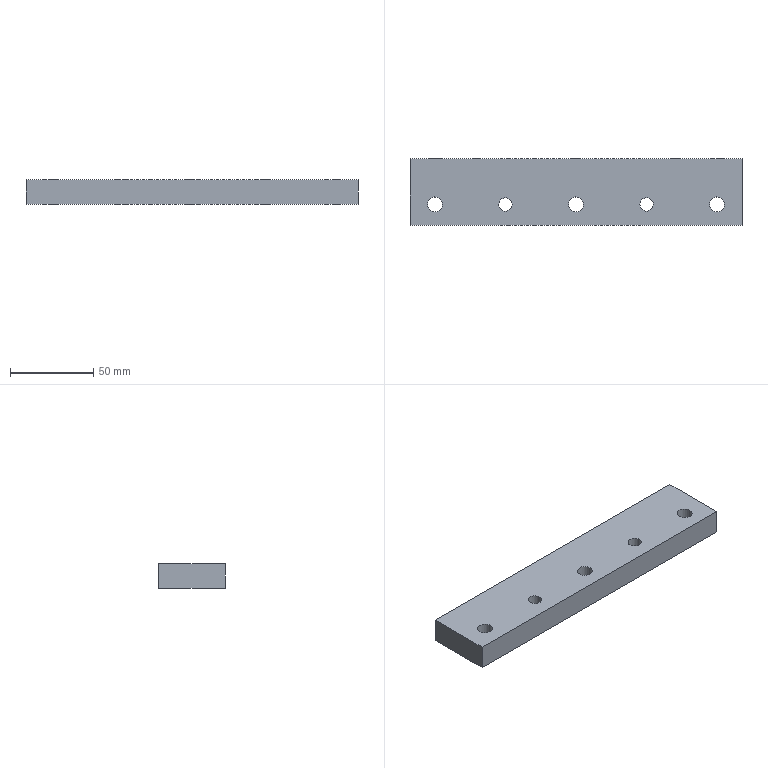Part | STEP file | SN10_001_002_SUPORTE | 1 solid | 21 faces | box 200 x 40 x 15 mm | volume 112660 mm3 | cylinder 10 | plane 6 | cone 5 | commonest cylinder face diameters 8 x4 4.917 x3 9 x3
STEP:
#1=CARTESIAN_POINT('',(0.,0.,0.));
#2=DIRECTION('',(0.,0.,1.));
#3=DIRECTION('',(1.,0.,0.));
#4=AXIS2_PLACEMENT_3D('',#1,#2,#3);
#5=CARTESIAN_POINT('',(-81.49,195.,59.418));
#6=VERTEX_POINT('',#5);
#7=CARTESIAN_POINT('',(-85.,195.,57.5));
#8=DIRECTION('',(0.,1.,0.));
#9=DIRECTION('',(1.,0.,0.));
#10=AXIS2_PLACEMENT_3D('',#7,#8,#9);
#11=CIRCLE('',#10,4.);
#12=CARTESIAN_POINT('',(-85.,193.268,57.5));
#13=DIRECTION('',(0.,1.,0.));
#14=DIRECTION('',(0.8776,0.,0.4794));
#15=AXIS2_PLACEMENT_3D('',#12,#13,#14);
#16=CONICAL_SURFACE('',#15,1.,1.047);
#17=CARTESIAN_POINT('',(-5.783,1.732));
#18=DIRECTION('',(1.,0.));
#19=VECTOR('',#18,1.);
#20=LINE('',#17,#19);
#21=(GEOMETRIC_REPRESENTATION_CONTEXT(2)PARAMETRIC_REPRESENTATION_CONTEXT()REPRESENTATION_CONTEXT('',''));
#22=DEFINITIONAL_REPRESENTATION('',(#20),#21);
#23=PCURVE('',#16,#22);
#24=CARTESIAN_POINT('',(-85.,214.9,57.5));
#25=DIRECTION('',(0.,-1.,0.));
#26=DIRECTION('',(0.8776,0.,0.4794));
#27=AXIS2_PLACEMENT_3D('',#24,#25,#26);
#28=CYLINDRICAL_SURFACE('',#27,4.);
#29=CARTESIAN_POINT('',(12.066,19.9));
#30=DIRECTION('',(-1.,0.));
#31=VECTOR('',#30,1.);
#32=LINE('',#29,#31);
#33=(GEOMETRIC_REPRESENTATION_CONTEXT(2)PARAMETRIC_REPRESENTATION_CONTEXT()REPRESENTATION_CONTEXT('',''));
#34=DEFINITIONAL_REPRESENTATION('',(#32),#33);
#35=PCURVE('',#28,#34);
#36=SURFACE_CURVE('',#11,(#23,#35),.PCURVE_S1.);
#37=EDGE_CURVE('',#6,#6,#36,.T.);
#38=ORIENTED_EDGE('',*,*,#37,.F.);
#39=CARTESIAN_POINT('',(-85.,192.691,57.5));
#40=VERTEX_POINT('',#39);
#41=CARTESIAN_POINT('',(-85.,192.691,57.5));
#42=CARTESIAN_POINT('',(-81.49,195.,59.418));
#43=B_SPLINE_CURVE_WITH_KNOTS('',1,(#41,#42),.UNSPECIFIED.,.F.,.F.,(2,2),(-1.155,3.464),.PIECEWISE_BEZIER_KNOTS.);
#44=CARTESIAN_POINT('',(0.,0.));
#45=DIRECTION('',(0.,1.));
#46=VECTOR('',#45,1.);
#47=LINE('',#44,#46);
#48=(GEOMETRIC_REPRESENTATION_CONTEXT(2)PARAMETRIC_REPRESENTATION_CONTEXT()REPRESENTATION_CONTEXT('',''));
#49=DEFINITIONAL_REPRESENTATION('',(#47),#48);
#50=PCURVE('',#16,#49);
#51=CARTESIAN_POINT('',(6.283,0.));
#52=DIRECTION('',(0.,1.));
#53=VECTOR('',#52,1.);
#54=LINE('',#51,#53);
#55=(GEOMETRIC_REPRESENTATION_CONTEXT(2)PARAMETRIC_REPRESENTATION_CONTEXT()REPRESENTATION_CONTEXT('',''));
#56=DEFINITIONAL_REPRESENTATION('',(#54),#55);
#57=PCURVE('',#16,#56);
#58=SEAM_CURVE('',#43,(#50,#57),.PCURVE_S1.);
#59=EDGE_CURVE('',#40,#6,#58,.T.);
#60=ORIENTED_EDGE('',*,*,#59,.F.);
#61=ORIENTED_EDGE('',*,*,#59,.T.);
#62=EDGE_LOOP('',(#38,#60,#61));
#63=FACE_BOUND('',#62,.F.);
#64=ADVANCED_FACE('',(#63),#16,.F.);
#65=CARTESIAN_POINT('',(-100.,215.,65.));
#66=VERTEX_POINT('',#65);
#67=CARTESIAN_POINT('',(100.,215.,65.));
#68=VERTEX_POINT('',#67);
#69=CARTESIAN_POINT('',(-100.,215.,65.));
#70=DIRECTION('',(1.,0.,0.));
#71=VECTOR('',#70,1.);
#72=LINE('',#69,#71);
#73=CARTESIAN_POINT('',(0.,175.,65.));
#74=DIRECTION('',(0.,0.,-1.));
#75=DIRECTION('',(-1.,0.,0.));
#76=AXIS2_PLACEMENT_3D('',#73,#74,#75);
#77=PLANE('',#76);
#78=CARTESIAN_POINT('',(100.,40.));
#79=DIRECTION('',(-1.,0.));
#80=VECTOR('',#79,1.);
#81=LINE('',#78,#80);
#82=(GEOMETRIC_REPRESENTATION_CONTEXT(2)PARAMETRIC_REPRESENTATION_CONTEXT()REPRESENTATION_CONTEXT('',''));
#83=DEFINITIONAL_REPRESENTATION('',(#81),#82);
#84=PCURVE('',#77,#83);
#85=CARTESIAN_POINT('',(0.,215.,65.));
#86=DIRECTION('',(0.,-1.,0.));
#87=DIRECTION('',(0.,0.,-1.));
#88=AXIS2_PLACEMENT_3D('',#85,#86,#87);
#89=PLANE('',#88);
#90=CARTESIAN_POINT('',(0.,-100.));
#91=DIRECTION('',(0.,1.));
#92=VECTOR('',#91,1.);
#93=LINE('',#90,#92);
#94=(GEOMETRIC_REPRESENTATION_CONTEXT(2)PARAMETRIC_REPRESENTATION_CONTEXT()REPRESENTATION_CONTEXT('',''));
#95=DEFINITIONAL_REPRESENTATION('',(#93),#94);
#96=PCURVE('',#89,#95);
#97=SURFACE_CURVE('',#72,(#84,#96),.PCURVE_S1.);
#98=EDGE_CURVE('',#66,#68,#97,.T.);
#99=ORIENTED_EDGE('',*,*,#98,.F.);
#100=CARTESIAN_POINT('',(-100.,175.,65.));
#101=VERTEX_POINT('',#100);
#102=CARTESIAN_POINT('',(-100.,175.,65.));
#103=DIRECTION('',(0.,1.,0.));
#104=VECTOR('',#103,1.);
#105=LINE('',#102,#104);
#106=CARTESIAN_POINT('',(100.,0.));
#107=DIRECTION('',(0.,1.));
#108=VECTOR('',#107,1.);
#109=LINE('',#106,#108);
#110=(GEOMETRIC_REPRESENTATION_CONTEXT(2)PARAMETRIC_REPRESENTATION_CONTEXT()REPRESENTATION_CONTEXT('',''));
#111=DEFINITIONAL_REPRESENTATION('',(#109),#110);
#112=PCURVE('',#77,#111);
#113=CARTESIAN_POINT('',(-100.,0.,0.));
#114=DIRECTION('',(1.,0.,0.));
#115=DIRECTION('',(0.,0.,-1.));
#116=AXIS2_PLACEMENT_3D('',#113,#114,#115);
#117=PLANE('',#116);
#118=CARTESIAN_POINT('',(-65.,175.));
#119=DIRECTION('',(0.,1.));
#120=VECTOR('',#119,1.);
#121=LINE('',#118,#120);
#122=(GEOMETRIC_REPRESENTATION_CONTEXT(2)PARAMETRIC_REPRESENTATION_CONTEXT()REPRESENTATION_CONTEXT('',''));
#123=DEFINITIONAL_REPRESENTATION('',(#121),#122);
#124=PCURVE('',#117,#123);
#125=SURFACE_CURVE('',#105,(#112,#124),.PCURVE_S1.);
#126=EDGE_CURVE('',#101,#66,#125,.T.);
#127=ORIENTED_EDGE('',*,*,#126,.F.);
#128=CARTESIAN_POINT('',(100.,175.,65.));
#129=VERTEX_POINT('',#128);
#130=CARTESIAN_POINT('',(-100.,175.,65.));
#131=DIRECTION('',(1.,0.,0.));
#132=VECTOR('',#131,1.);
#133=LINE('',#130,#132);
#134=CARTESIAN_POINT('',(100.,0.));
#135=DIRECTION('',(-1.,0.));
#136=VECTOR('',#135,1.);
#137=LINE('',#134,#136);
#138=(GEOMETRIC_REPRESENTATION_CONTEXT(2)PARAMETRIC_REPRESENTATION_CONTEXT()REPRESENTATION_CONTEXT('',''));
#139=DEFINITIONAL_REPRESENTATION('',(#137),#138);
#140=PCURVE('',#77,#139);
#141=CARTESIAN_POINT('',(0.,175.,50.));
#142=DIRECTION('',(0.,1.,0.));
#143=DIRECTION('',(0.,0.,1.));
#144=AXIS2_PLACEMENT_3D('',#141,#142,#143);
#145=PLANE('',#144);
#146=CARTESIAN_POINT('',(15.,-100.));
#147=DIRECTION('',(0.,1.));
#148=VECTOR('',#147,1.);
#149=LINE('',#146,#148);
#150=(GEOMETRIC_REPRESENTATION_CONTEXT(2)PARAMETRIC_REPRESENTATION_CONTEXT()REPRESENTATION_CONTEXT('',''));
#151=DEFINITIONAL_REPRESENTATION('',(#149),#150);
#152=PCURVE('',#145,#151);
#153=SURFACE_CURVE('',#133,(#140,#152),.PCURVE_S1.);
#154=EDGE_CURVE('',#101,#129,#153,.T.);
#155=ORIENTED_EDGE('',*,*,#154,.T.);
#156=CARTESIAN_POINT('',(100.,175.,65.));
#157=DIRECTION('',(0.,1.,0.));
#158=VECTOR('',#157,1.);
#159=LINE('',#156,#158);
#160=CARTESIAN_POINT('',(-100.,0.));
#161=DIRECTION('',(0.,1.));
#162=VECTOR('',#161,1.);
#163=LINE('',#160,#162);
#164=(GEOMETRIC_REPRESENTATION_CONTEXT(2)PARAMETRIC_REPRESENTATION_CONTEXT()REPRESENTATION_CONTEXT('',''));
#165=DEFINITIONAL_REPRESENTATION('',(#163),#164);
#166=PCURVE('',#77,#165);
#167=CARTESIAN_POINT('',(100.,0.,0.));
#168=DIRECTION('',(1.,0.,0.));
#169=DIRECTION('',(0.,0.,-1.));
#170=AXIS2_PLACEMENT_3D('',#167,#168,#169);
#171=PLANE('',#170);
#172=CARTESIAN_POINT('',(-65.,175.));
#173=DIRECTION('',(0.,1.));
#174=VECTOR('',#173,1.);
#175=LINE('',#172,#174);
#176=(GEOMETRIC_REPRESENTATION_CONTEXT(2)PARAMETRIC_REPRESENTATION_CONTEXT()REPRESENTATION_CONTEXT('',''));
#177=DEFINITIONAL_REPRESENTATION('',(#175),#176);
#178=PCURVE('',#171,#177);
#179=SURFACE_CURVE('',#159,(#166,#178),.PCURVE_S1.);
#180=EDGE_CURVE('',#129,#68,#179,.T.);
#181=ORIENTED_EDGE('',*,*,#180,.T.);
#182=EDGE_LOOP('',(#99,#127,#155,#181));
#183=FACE_BOUND('',#182,.T.);
#184=CARTESIAN_POINT('',(38.99,189.418,65.));
#185=VERTEX_POINT('',#184);
#186=CARTESIAN_POINT('',(42.5,187.5,65.));
#187=DIRECTION('',(0.,0.,-1.));
#188=DIRECTION('',(1.,0.,0.));
#189=AXIS2_PLACEMENT_3D('',#186,#187,#188);
#190=CIRCLE('',#189,4.);
#191=CARTESIAN_POINT('',(-42.5,12.5));
#192=DIRECTION('',(-1.,0.));
#193=AXIS2_PLACEMENT_2D('',#191,#192);
#194=CIRCLE('',#193,4.);
#195=(GEOMETRIC_REPRESENTATION_CONTEXT(2)PARAMETRIC_REPRESENTATION_CONTEXT()REPRESENTATION_CONTEXT('',''));
#196=DEFINITIONAL_REPRESENTATION('',(#194),#195);
#197=PCURVE('',#77,#196);
#198=CARTESIAN_POINT('',(42.5,187.5,64.9));
#199=DIRECTION('',(0.,0.,-1.));
#200=DIRECTION('',(0.8776,-0.4794,0.));
#201=AXIS2_PLACEMENT_3D('',#198,#199,#200);
#202=CYLINDRICAL_SURFACE('',#201,4.);
#203=CARTESIAN_POINT('',(-0.5,-0.1));
#204=DIRECTION('',(1.,0.));
#205=VECTOR('',#204,1.);
#206=LINE('',#203,#205);
#207=(GEOMETRIC_REPRESENTATION_CONTEXT(2)PARAMETRIC_REPRESENTATION_CONTEXT()REPRESENTATION_CONTEXT('',''));
#208=DEFINITIONAL_REPRESENTATION('',(#206),#207);
#209=PCURVE('',#202,#208);
#210=SURFACE_CURVE('',#190,(#197,#209),.PCURVE_S1.);
#211=EDGE_CURVE('',#185,#185,#210,.T.);
#212=ORIENTED_EDGE('',*,*,#211,.T.);
#213=EDGE_LOOP('',(#212));
#214=FACE_BOUND('',#213,.T.);
#215=CARTESIAN_POINT('',(-46.01,189.418,65.));
#216=VERTEX_POINT('',#215);
#217=CARTESIAN_POINT('',(-42.5,187.5,65.));
#218=DIRECTION('',(0.,0.,-1.));
#219=DIRECTION('',(1.,0.,0.));
#220=AXIS2_PLACEMENT_3D('',#217,#218,#219);
#221=CIRCLE('',#220,4.);
#222=CARTESIAN_POINT('',(42.5,12.5));
#223=DIRECTION('',(-1.,0.));
#224=AXIS2_PLACEMENT_2D('',#222,#223);
#225=CIRCLE('',#224,4.);
#226=(GEOMETRIC_REPRESENTATION_CONTEXT(2)PARAMETRIC_REPRESENTATION_CONTEXT()REPRESENTATION_CONTEXT('',''));
#227=DEFINITIONAL_REPRESENTATION('',(#225),#226);
#228=PCURVE('',#77,#227);
#229=CARTESIAN_POINT('',(-42.5,187.5,64.9));
#230=DIRECTION('',(0.,0.,-1.));
#231=DIRECTION('',(0.8776,-0.4794,0.));
#232=AXIS2_PLACEMENT_3D('',#229,#230,#231);
#233=CYLINDRICAL_SURFACE('',#232,4.);
#234=CARTESIAN_POINT('',(-0.5,-0.1));
#235=DIRECTION('',(1.,0.));
#236=VECTOR('',#235,1.);
#237=LINE('',#234,#236);
#238=(GEOMETRIC_REPRESENTATION_CONTEXT(2)PARAMETRIC_REPRESENTATION_CONTEXT()REPRESENTATION_CONTEXT('',''));
#239=DEFINITIONAL_REPRESENTATION('',(#237),#238);
#240=PCURVE('',#233,#239);
#241=SURFACE_CURVE('',#221,(#228,#240),.PCURVE_S1.);
#242=EDGE_CURVE('',#216,#216,#241,.T.);
#243=ORIENTED_EDGE('',*,*,#242,.T.);
#244=EDGE_LOOP('',(#243));
#245=FACE_BOUND('',#244,.T.);
#246=CARTESIAN_POINT('',(-88.949,189.657,65.));
#247=VERTEX_POINT('',#246);
#248=CARTESIAN_POINT('',(-85.,187.5,65.));
#249=DIRECTION('',(0.,0.,-1.));
#250=DIRECTION('',(1.,0.,0.));
#251=AXIS2_PLACEMENT_3D('',#248,#249,#250);
#252=CIRCLE('',#251,4.5);
#253=CARTESIAN_POINT('',(85.,12.5));
#254=DIRECTION('',(-1.,0.));
#255=AXIS2_PLACEMENT_2D('',#253,#254);
#256=CIRCLE('',#255,4.5);
#257=(GEOMETRIC_REPRESENTATION_CONTEXT(2)PARAMETRIC_REPRESENTATION_CONTEXT()REPRESENTATION_CONTEXT('',''));
#258=DEFINITIONAL_REPRESENTATION('',(#256),#257);
#259=PCURVE('',#77,#258);
#260=CARTESIAN_POINT('',(-85.,187.5,64.9));
#261=DIRECTION('',(0.,0.,-1.));
#262=DIRECTION('',(0.8776,-0.4794,0.));
#263=AXIS2_PLACEMENT_3D('',#260,#261,#262);
#264=CYLINDRICAL_SURFACE('',#263,4.5);
#265=CARTESIAN_POINT('',(-0.5,-0.1));
#266=DIRECTION('',(1.,0.));
#267=VECTOR('',#266,1.);
#268=LINE('',#265,#267);
#269=(GEOMETRIC_REPRESENTATION_CONTEXT(2)PARAMETRIC_REPRESENTATION_CONTEXT()REPRESENTATION_CONTEXT('',''));
#270=DEFINITIONAL_REPRESENTATION('',(#268),#269);
#271=PCURVE('',#264,#270);
#272=SURFACE_CURVE('',#252,(#259,#271),.PCURVE_S1.);
#273=EDGE_CURVE('',#247,#247,#272,.T.);
#274=ORIENTED_EDGE('',*,*,#273,.T.);
#275=EDGE_LOOP('',(#274));
#276=FACE_BOUND('',#275,.T.);
#277=CARTESIAN_POINT('',(-3.949,189.657,65.));
#278=VERTEX_POINT('',#277);
#279=CARTESIAN_POINT('',(0.,187.5,65.));
#280=DIRECTION('',(0.,0.,-1.));
#281=DIRECTION('',(1.,0.,0.));
#282=AXIS2_PLACEMENT_3D('',#279,#280,#281);
#283=CIRCLE('',#282,4.5);
#284=CARTESIAN_POINT('',(0.,12.5));
#285=DIRECTION('',(-1.,0.));
#286=AXIS2_PLACEMENT_2D('',#284,#285);
#287=CIRCLE('',#286,4.5);
#288=(GEOMETRIC_REPRESENTATION_CONTEXT(2)PARAMETRIC_REPRESENTATION_CONTEXT()REPRESENTATION_CONTEXT('',''));
#289=DEFINITIONAL_REPRESENTATION('',(#287),#288);
#290=PCURVE('',#77,#289);
#291=CARTESIAN_POINT('',(0.,187.5,64.9));
#292=DIRECTION('',(0.,0.,-1.));
#293=DIRECTION('',(0.8776,-0.4794,0.));
#294=AXIS2_PLACEMENT_3D('',#291,#292,#293);
#295=CYLINDRICAL_SURFACE('',#294,4.5);
#296=CARTESIAN_POINT('',(-0.5,-0.1));
#297=DIRECTION('',(1.,0.));
#298=VECTOR('',#297,1.);
#299=LINE('',#296,#298);
#300=(GEOMETRIC_REPRESENTATION_CONTEXT(2)PARAMETRIC_REPRESENTATION_CONTEXT()REPRESENTATION_CONTEXT('',''));
#301=DEFINITIONAL_REPRESENTATION('',(#299),#300);
#302=PCURVE('',#295,#301);
#303=SURFACE_CURVE('',#283,(#290,#302),.PCURVE_S1.);
#304=EDGE_CURVE('',#278,#278,#303,.T.);
#305=ORIENTED_EDGE('',*,*,#304,.T.);
#306=EDGE_LOOP('',(#305));
#307=FACE_BOUND('',#306,.T.);
#308=CARTESIAN_POINT('',(81.051,189.657,65.));
#309=VERTEX_POINT('',#308);
#310=CARTESIAN_POINT('',(85.,187.5,65.));
#311=DIRECTION('',(0.,0.,-1.));
#312=DIRECTION('',(1.,0.,0.));
#313=AXIS2_PLACEMENT_3D('',#310,#311,#312);
#314=CIRCLE('',#313,4.5);
#315=CARTESIAN_POINT('',(-85.,12.5));
#316=DIRECTION('',(-1.,0.));
#317=AXIS2_PLACEMENT_2D('',#315,#316);
#318=CIRCLE('',#317,4.5);
#319=(GEOMETRIC_REPRESENTATION_CONTEXT(2)PARAMETRIC_REPRESENTATION_CONTEXT()REPRESENTATION_CONTEXT('',''));
#320=DEFINITIONAL_REPRESENTATION('',(#318),#319);
#321=PCURVE('',#77,#320);
#322=CARTESIAN_POINT('',(85.,187.5,64.9));
#323=DIRECTION('',(0.,0.,-1.));
#324=DIRECTION('',(0.8776,-0.4794,0.));
#325=AXIS2_PLACEMENT_3D('',#322,#323,#324);
#326=CYLINDRICAL_SURFACE('',#325,4.5);
#327=CARTESIAN_POINT('',(-0.5,-0.1));
#328=DIRECTION('',(1.,0.));
#329=VECTOR('',#328,1.);
#330=LINE('',#327,#329);
#331=(GEOMETRIC_REPRESENTATION_CONTEXT(2)PARAMETRIC_REPRESENTATION_CONTEXT()REPRESENTATION_CONTEXT('',''));
#332=DEFINITIONAL_REPRESENTATION('',(#330),#331);
#333=PCURVE('',#326,#332);
#334=SURFACE_CURVE('',#314,(#321,#333),.PCURVE_S1.);
#335=EDGE_CURVE('',#309,#309,#334,.T.);
#336=ORIENTED_EDGE('',*,*,#335,.T.);
#337=EDGE_LOOP('',(#336));
#338=FACE_BOUND('',#337,.T.);
#339=ADVANCED_FACE('',(#183,#214,#245,#276,#307,#338),#77,.F.);
#340=CARTESIAN_POINT('',(-100.,215.,50.));
#341=VERTEX_POINT('',#340);
#342=CARTESIAN_POINT('',(-100.,215.,65.));
#343=DIRECTION('',(0.,0.,-1.));
#344=VECTOR('',#343,1.);
#345=LINE('',#342,#344);
#346=CARTESIAN_POINT('',(-65.,215.));
#347=DIRECTION('',(1.,0.));
#348=VECTOR('',#347,1.);
#349=LINE('',#346,#348);
#350=(GEOMETRIC_REPRESENTATION_CONTEXT(2)PARAMETRIC_REPRESENTATION_CONTEXT()REPRESENTATION_CONTEXT('',''));
#351=DEFINITIONAL_REPRESENTATION('',(#349),#350);
#352=PCURVE('',#117,#351);
#353=CARTESIAN_POINT('',(0.,-100.));
#354=DIRECTION('',(1.,0.));
#355=VECTOR('',#354,1.);
#356=LINE('',#353,#355);
#357=(GEOMETRIC_REPRESENTATION_CONTEXT(2)PARAMETRIC_REPRESENTATION_CONTEXT()REPRESENTATION_CONTEXT('',''));
#358=DEFINITIONAL_REPRESENTATION('',(#356),#357);
#359=PCURVE('',#89,#358);
#360=SURFACE_CURVE('',#345,(#352,#359),.PCURVE_S1.);
#361=EDGE_CURVE('',#66,#341,#360,.T.);
#362=ORIENTED_EDGE('',*,*,#361,.T.);
#363=CARTESIAN_POINT('',(-100.,175.,50.));
#364=VERTEX_POINT('',#363);
#365=CARTESIAN_POINT('',(-100.,215.,50.));
#366=DIRECTION('',(0.,-1.,0.));
#367=VECTOR('',#366,1.);
#368=LINE('',#365,#367);
#369=CARTESIAN_POINT('',(-50.,215.));
#370=DIRECTION('',(0.,-1.));
#371=VECTOR('',#370,1.);
#372=LINE('',#369,#371);
#373=(GEOMETRIC_REPRESENTATION_CONTEXT(2)PARAMETRIC_REPRESENTATION_CONTEXT()REPRESENTATION_CONTEXT('',''));
#374=DEFINITIONAL_REPRESENTATION('',(#372),#373);
#375=PCURVE('',#117,#374);
#376=CARTESIAN_POINT('',(0.,215.,50.));
#377=DIRECTION('',(0.,0.,1.));
#378=DIRECTION('',(1.,0.,0.));
#379=AXIS2_PLACEMENT_3D('',#376,#377,#378);
#380=PLANE('',#379);
#381=CARTESIAN_POINT('',(-100.,0.));
#382=DIRECTION('',(0.,-1.));
#383=VECTOR('',#382,1.);
#384=LINE('',#381,#383);
#385=(GEOMETRIC_REPRESENTATION_CONTEXT(2)PARAMETRIC_REPRESENTATION_CONTEXT()REPRESENTATION_CONTEXT('',''));
#386=DEFINITIONAL_REPRESENTATION('',(#384),#385);
#387=PCURVE('',#380,#386);
#388=SURFACE_CURVE('',#368,(#375,#387),.PCURVE_S1.);
#389=EDGE_CURVE('',#341,#364,#388,.T.);
#390=ORIENTED_EDGE('',*,*,#389,.T.);
#391=CARTESIAN_POINT('',(-100.,175.,50.));
#392=DIRECTION('',(0.,0.,1.));
#393=VECTOR('',#392,1.);
#394=LINE('',#391,#393);
#395=CARTESIAN_POINT('',(-50.,175.));
#396=DIRECTION('',(-1.,0.));
#397=VECTOR('',#396,1.);
#398=LINE('',#395,#397);
#399=(GEOMETRIC_REPRESENTATION_CONTEXT(2)PARAMETRIC_REPRESENTATION_CONTEXT()REPRESENTATION_CONTEXT('',''));
#400=DEFINITIONAL_REPRESENTATION('',(#398),#399);
#401=PCURVE('',#117,#400);
#402=CARTESIAN_POINT('',(0.,-100.));
#403=DIRECTION('',(1.,0.));
#404=VECTOR('',#403,1.);
#405=LINE('',#402,#404);
#406=(GEOMETRIC_REPRESENTATION_CONTEXT(2)PARAMETRIC_REPRESENTATION_CONTEXT()REPRESENTATION_CONTEXT('',''));
#407=DEFINITIONAL_REPRESENTATION('',(#405),#406);
#408=PCURVE('',#145,#407);
#409=SURFACE_CURVE('',#394,(#401,#408),.PCURVE_S1.);
#410=EDGE_CURVE('',#364,#101,#409,.T.);
#411=ORIENTED_EDGE('',*,*,#410,.T.);
#412=ORIENTED_EDGE('',*,*,#126,.T.);
#413=EDGE_LOOP('',(#362,#390,#411,#412));
#414=FACE_BOUND('',#413,.T.);
#415=ADVANCED_FACE('',(#414),#117,.F.);
#416=CARTESIAN_POINT('',(81.49,215.,55.582));
#417=VERTEX_POINT('',#416);
#418=CARTESIAN_POINT('',(85.,215.,57.5));
#419=DIRECTION('',(0.,-1.,0.));
#420=DIRECTION('',(1.,0.,0.));
#421=AXIS2_PLACEMENT_3D('',#418,#419,#420);
#422=CIRCLE('',#421,4.);
#423=CARTESIAN_POINT('',(85.,214.9,57.5));
#424=DIRECTION('',(0.,-1.,0.));
#425=DIRECTION('',(0.8776,0.,0.4794));
#426=AXIS2_PLACEMENT_3D('',#423,#424,#425);
#427=CYLINDRICAL_SURFACE('',#426,4.);
#428=CARTESIAN_POINT('',(-0.5,-0.1));
#429=DIRECTION('',(1.,0.));
#430=VECTOR('',#429,1.);
#431=LINE('',#428,#430);
#432=(GEOMETRIC_REPRESENTATION_CONTEXT(2)PARAMETRIC_REPRESENTATION_CONTEXT()REPRESENTATION_CONTEXT('',''));
#433=DEFINITIONAL_REPRESENTATION('',(#431),#432);
#434=PCURVE('',#427,#433);
#435=CARTESIAN_POINT('',(7.5,85.));
#436=DIRECTION('',(0.,1.));
#437=AXIS2_PLACEMENT_2D('',#435,#436);
#438=CIRCLE('',#437,4.);
#439=(GEOMETRIC_REPRESENTATION_CONTEXT(2)PARAMETRIC_REPRESENTATION_CONTEXT()REPRESENTATION_CONTEXT('',''));
#440=DEFINITIONAL_REPRESENTATION('',(#438),#439);
#441=PCURVE('',#89,#440);
#442=SURFACE_CURVE('',#422,(#434,#441),.PCURVE_S1.);
#443=EDGE_CURVE('',#417,#417,#442,.T.);
#444=ORIENTED_EDGE('',*,*,#443,.T.);
#445=CARTESIAN_POINT('',(81.49,195.,55.582));
#446=VERTEX_POINT('',#445);
#447=CARTESIAN_POINT('',(81.49,215.,55.582));
#448=CARTESIAN_POINT('',(81.49,195.,55.582));
#449=B_SPLINE_CURVE_WITH_KNOTS('',1,(#447,#448),.UNSPECIFIED.,.F.,.F.,(2,2),(-0.1,19.9),.PIECEWISE_BEZIER_KNOTS.);
#450=CARTESIAN_POINT('',(9.425,0.));
#451=DIRECTION('',(0.,1.));
#452=VECTOR('',#451,1.);
#453=LINE('',#450,#452);
#454=(GEOMETRIC_REPRESENTATION_CONTEXT(2)PARAMETRIC_REPRESENTATION_CONTEXT()REPRESENTATION_CONTEXT('',''));
#455=DEFINITIONAL_REPRESENTATION('',(#453),#454);
#456=PCURVE('',#427,#455);
#457=CARTESIAN_POINT('',(3.142,0.));
#458=DIRECTION('',(0.,1.));
#459=VECTOR('',#458,1.);
#460=LINE('',#457,#459);
#461=(GEOMETRIC_REPRESENTATION_CONTEXT(2)PARAMETRIC_REPRESENTATION_CONTEXT()REPRESENTATION_CONTEXT('',''));
#462=DEFINITIONAL_REPRESENTATION('',(#460),#461);
#463=PCURVE('',#427,#462);
#464=SEAM_CURVE('',#449,(#456,#463),.PCURVE_S1.);
#465=EDGE_CURVE('',#417,#446,#464,.T.);
#466=ORIENTED_EDGE('',*,*,#465,.T.);
#467=CARTESIAN_POINT('',(85.,195.,57.5));
#468=DIRECTION('',(0.,-1.,0.));
#469=DIRECTION('',(1.,0.,0.));
#470=AXIS2_PLACEMENT_3D('',#467,#468,#469);
#471=CIRCLE('',#470,4.);
#472=CARTESIAN_POINT('',(-0.5,19.9));
#473=DIRECTION('',(1.,0.));
#474=VECTOR('',#473,1.);
#475=LINE('',#472,#474);
#476=(GEOMETRIC_REPRESENTATION_CONTEXT(2)PARAMETRIC_REPRESENTATION_CONTEXT()REPRESENTATION_CONTEXT('',''));
#477=DEFINITIONAL_REPRESENTATION('',(#475),#476);
#478=PCURVE('',#427,#477);
#479=CARTESIAN_POINT('',(85.,193.268,57.5));
#480=DIRECTION('',(0.,1.,0.));
#481=DIRECTION('',(0.8776,0.,0.4794));
#482=AXIS2_PLACEMENT_3D('',#479,#480,#481);
#483=CONICAL_SURFACE('',#482,1.,1.047);
#484=CARTESIAN_POINT('',(13.066,1.732));
#485=DIRECTION('',(-1.,0.));
#486=VECTOR('',#485,1.);
#487=LINE('',#484,#486);
#488=(GEOMETRIC_REPRESENTATION_CONTEXT(2)PARAMETRIC_REPRESENTATION_CONTEXT()REPRESENTATION_CONTEXT('',''));
#489=DEFINITIONAL_REPRESENTATION('',(#487),#488);
#490=PCURVE('',#483,#489);
#491=SURFACE_CURVE('',#471,(#478,#490),.PCURVE_S1.);
#492=EDGE_CURVE('',#446,#446,#491,.T.);
#493=ORIENTED_EDGE('',*,*,#492,.F.);
#494=ORIENTED_EDGE('',*,*,#465,.F.);
#495=EDGE_LOOP('',(#444,#466,#493,#494));
#496=FACE_BOUND('',#495,.F.);
#497=ADVANCED_FACE('',(#496),#427,.F.);
#498=CARTESIAN_POINT('',(-62.158,215.,56.321));
#499=VERTEX_POINT('',#498);
#500=CARTESIAN_POINT('',(-60.,215.,57.5));
#501=DIRECTION('',(0.,-1.,0.));
#502=DIRECTION('',(1.,0.,0.));
#503=AXIS2_PLACEMENT_3D('',#500,#501,#502);
#504=CIRCLE('',#503,2.458);
#505=CARTESIAN_POINT('',(-60.,214.9,57.5));
#506=DIRECTION('',(0.,-1.,0.));
#507=DIRECTION('',(0.8776,0.,0.4794));
#508=AXIS2_PLACEMENT_3D('',#505,#506,#507);
#509=CYLINDRICAL_SURFACE('',#508,2.458);
#510=CARTESIAN_POINT('',(-0.5,-0.1));
#511=DIRECTION('',(1.,0.));
#512=VECTOR('',#511,1.);
#513=LINE('',#510,#512);
#514=(GEOMETRIC_REPRESENTATION_CONTEXT(2)PARAMETRIC_REPRESENTATION_CONTEXT()REPRESENTATION_CONTEXT('',''));
#515=DEFINITIONAL_REPRESENTATION('',(#513),#514);
#516=PCURVE('',#509,#515);
#517=CARTESIAN_POINT('',(7.5,-60.));
#518=DIRECTION('',(0.,1.));
#519=AXIS2_PLACEMENT_2D('',#517,#518);
#520=CIRCLE('',#519,2.458);
#521=(GEOMETRIC_REPRESENTATION_CONTEXT(2)PARAMETRIC_REPRESENTATION_CONTEXT()REPRESENTATION_CONTEXT('',''));
#522=DEFINITIONAL_REPRESENTATION('',(#520),#521);
#523=PCURVE('',#89,#522);
#524=SURFACE_CURVE('',#504,(#516,#523),.PCURVE_S1.);
#525=EDGE_CURVE('',#499,#499,#524,.T.);
#526=ORIENTED_EDGE('',*,*,#525,.T.);
#527=CARTESIAN_POINT('',(-62.158,200.,56.321));
#528=VERTEX_POINT('',#527);
#529=CARTESIAN_POINT('',(-62.158,215.,56.321));
#530=CARTESIAN_POINT('',(-62.158,200.,56.321));
#531=B_SPLINE_CURVE_WITH_KNOTS('',1,(#529,#530),.UNSPECIFIED.,.F.,.F.,(2,2),(-0.1,14.9),.PIECEWISE_BEZIER_KNOTS.);
#532=CARTESIAN_POINT('',(9.425,0.));
#533=DIRECTION('',(0.,1.));
#534=VECTOR('',#533,1.);
#535=LINE('',#532,#534);
#536=(GEOMETRIC_REPRESENTATION_CONTEXT(2)PARAMETRIC_REPRESENTATION_CONTEXT()REPRESENTATION_CONTEXT('',''));
#537=DEFINITIONAL_REPRESENTATION('',(#535),#536);
#538=PCURVE('',#509,#537);
#539=CARTESIAN_POINT('',(3.142,0.));
#540=DIRECTION('',(0.,1.));
#541=VECTOR('',#540,1.);
#542=LINE('',#539,#541);
#543=(GEOMETRIC_REPRESENTATION_CONTEXT(2)PARAMETRIC_REPRESENTATION_CONTEXT()REPRESENTATION_CONTEXT('',''));
#544=DEFINITIONAL_REPRESENTATION('',(#542),#543);
#545=PCURVE('',#509,#544);
#546=SEAM_CURVE('',#531,(#538,#545),.PCURVE_S1.);
#547=EDGE_CURVE('',#499,#528,#546,.T.);
#548=ORIENTED_EDGE('',*,*,#547,.T.);
#549=CARTESIAN_POINT('',(-60.,200.,57.5));
#550=DIRECTION('',(0.,-1.,0.));
#551=DIRECTION('',(1.,0.,0.));
#552=AXIS2_PLACEMENT_3D('',#549,#550,#551);
#553=CIRCLE('',#552,2.458);
#554=CARTESIAN_POINT('',(-0.5,14.9));
#555=DIRECTION('',(1.,0.));
#556=VECTOR('',#555,1.);
#557=LINE('',#554,#556);
#558=(GEOMETRIC_REPRESENTATION_CONTEXT(2)PARAMETRIC_REPRESENTATION_CONTEXT()REPRESENTATION_CONTEXT('',''));
#559=DEFINITIONAL_REPRESENTATION('',(#557),#558);
#560=PCURVE('',#509,#559);
#561=CARTESIAN_POINT('',(-60.,199.158,57.5));
#562=DIRECTION('',(0.,1.,0.));
#563=DIRECTION('',(0.8776,0.,0.4794));
#564=AXIS2_PLACEMENT_3D('',#561,#562,#563);
#565=CONICAL_SURFACE('',#564,1.,1.047);
#566=CARTESIAN_POINT('',(13.066,0.8421));
#567=DIRECTION('',(-1.,0.));
#568=VECTOR('',#567,1.);
#569=LINE('',#566,#568);
#570=(GEOMETRIC_REPRESENTATION_CONTEXT(2)PARAMETRIC_REPRESENTATION_CONTEXT()REPRESENTATION_CONTEXT('',''));
#571=DEFINITIONAL_REPRESENTATION('',(#569),#570);
#572=PCURVE('',#565,#571);
#573=SURFACE_CURVE('',#553,(#560,#572),.PCURVE_S1.);
#574=EDGE_CURVE('',#528,#528,#573,.T.);
#575=ORIENTED_EDGE('',*,*,#574,.F.);
#576=ORIENTED_EDGE('',*,*,#547,.F.);
#577=EDGE_LOOP('',(#526,#548,#575,#576));
#578=FACE_BOUND('',#577,.F.);
#579=ADVANCED_FACE('',(#578),#509,.F.);
#580=CARTESIAN_POINT('',(-2.158,215.,56.321));
#581=VERTEX_POINT('',#580);
#582=CARTESIAN_POINT('',(0.,215.,57.5));
#583=DIRECTION('',(0.,-1.,0.));
#584=DIRECTION('',(1.,0.,0.));
#585=AXIS2_PLACEMENT_3D('',#582,#583,#584);
#586=CIRCLE('',#585,2.458);
#587=CARTESIAN_POINT('',(0.,214.9,57.5));
#588=DIRECTION('',(0.,-1.,0.));
#589=DIRECTION('',(0.8776,0.,0.4794));
#590=AXIS2_PLACEMENT_3D('',#587,#588,#589);
#591=CYLINDRICAL_SURFACE('',#590,2.458);
#592=CARTESIAN_POINT('',(-0.5,-0.1));
#593=DIRECTION('',(1.,0.));
#594=VECTOR('',#593,1.);
#595=LINE('',#592,#594);
#596=(GEOMETRIC_REPRESENTATION_CONTEXT(2)PARAMETRIC_REPRESENTATION_CONTEXT()REPRESENTATION_CONTEXT('',''));
#597=DEFINITIONAL_REPRESENTATION('',(#595),#596);
#598=PCURVE('',#591,#597);
#599=CARTESIAN_POINT('',(7.5,0.));
#600=DIRECTION('',(0.,1.));
#601=AXIS2_PLACEMENT_2D('',#599,#600);
#602=CIRCLE('',#601,2.458);
#603=(GEOMETRIC_REPRESENTATION_CONTEXT(2)PARAMETRIC_REPRESENTATION_CONTEXT()REPRESENTATION_CONTEXT('',''));
#604=DEFINITIONAL_REPRESENTATION('',(#602),#603);
#605=PCURVE('',#89,#604);
#606=SURFACE_CURVE('',#586,(#598,#605),.PCURVE_S1.);
#607=EDGE_CURVE('',#581,#581,#606,.T.);
#608=ORIENTED_EDGE('',*,*,#607,.T.);
#609=CARTESIAN_POINT('',(-2.158,200.,56.321));
#610=VERTEX_POINT('',#609);
#611=CARTESIAN_POINT('',(-2.158,215.,56.321));
#612=CARTESIAN_POINT('',(-2.158,200.,56.321));
#613=B_SPLINE_CURVE_WITH_KNOTS('',1,(#611,#612),.UNSPECIFIED.,.F.,.F.,(2,2),(-0.1,14.9),.PIECEWISE_BEZIER_KNOTS.);
#614=CARTESIAN_POINT('',(9.425,0.));
#615=DIRECTION('',(0.,1.));
#616=VECTOR('',#615,1.);
#617=LINE('',#614,#616);
#618=(GEOMETRIC_REPRESENTATION_CONTEXT(2)PARAMETRIC_REPRESENTATION_CONTEXT()REPRESENTATION_CONTEXT('',''));
#619=DEFINITIONAL_REPRESENTATION('',(#617),#618);
#620=PCURVE('',#591,#619);
#621=CARTESIAN_POINT('',(3.142,0.));
#622=DIRECTION('',(0.,1.));
#623=VECTOR('',#622,1.);
#624=LINE('',#621,#623);
#625=(GEOMETRIC_REPRESENTATION_CONTEXT(2)PARAMETRIC_REPRESENTATION_CONTEXT()REPRESENTATION_CONTEXT('',''));
#626=DEFINITIONAL_REPRESENTATION('',(#624),#625);
#627=PCURVE('',#591,#626);
#628=SEAM_CURVE('',#613,(#620,#627),.PCURVE_S1.);
#629=EDGE_CURVE('',#581,#610,#628,.T.);
#630=ORIENTED_EDGE('',*,*,#629,.T.);
#631=CARTESIAN_POINT('',(0.,200.,57.5));
#632=DIRECTION('',(0.,-1.,0.));
#633=DIRECTION('',(1.,0.,0.));
#634=AXIS2_PLACEMENT_3D('',#631,#632,#633);
#635=CIRCLE('',#634,2.458);
#636=CARTESIAN_POINT('',(-0.5,14.9));
#637=DIRECTION('',(1.,0.));
#638=VECTOR('',#637,1.);
#639=LINE('',#636,#638);
#640=(GEOMETRIC_REPRESENTATION_CONTEXT(2)PARAMETRIC_REPRESENTATION_CONTEXT()REPRESENTATION_CONTEXT('',''));
#641=DEFINITIONAL_REPRESENTATION('',(#639),#640);
#642=PCURVE('',#591,#641);
#643=CARTESIAN_POINT('',(0.,199.158,57.5));
#644=DIRECTION('',(0.,1.,0.));
#645=DIRECTION('',(0.8776,0.,0.4794));
#646=AXIS2_PLACEMENT_3D('',#643,#644,#645);
#647=CONICAL_SURFACE('',#646,1.,1.047);
#648=CARTESIAN_POINT('',(13.066,0.8421));
#649=DIRECTION('',(-1.,0.));
#650=VECTOR('',#649,1.);
#651=LINE('',#648,#650);
#652=(GEOMETRIC_REPRESENTATION_CONTEXT(2)PARAMETRIC_REPRESENTATION_CONTEXT()REPRESENTATION_CONTEXT('',''));
#653=DEFINITIONAL_REPRESENTATION('',(#651),#652);
#654=PCURVE('',#647,#653);
#655=SURFACE_CURVE('',#635,(#642,#654),.PCURVE_S1.);
#656=EDGE_CURVE('',#610,#610,#655,.T.);
#657=ORIENTED_EDGE('',*,*,#656,.F.);
#658=ORIENTED_EDGE('',*,*,#629,.F.);
#659=EDGE_LOOP('',(#608,#630,#657,#658));
#660=FACE_BOUND('',#659,.F.);
#661=ADVANCED_FACE('',(#660),#591,.F.);
#662=CARTESIAN_POINT('',(57.842,215.,56.321));
#663=VERTEX_POINT('',#662);
#664=CARTESIAN_POINT('',(60.,215.,57.5));
#665=DIRECTION('',(0.,-1.,0.));
#666=DIRECTION('',(1.,0.,0.));
#667=AXIS2_PLACEMENT_3D('',#664,#665,#666);
#668=CIRCLE('',#667,2.458);
#669=CARTESIAN_POINT('',(60.,214.9,57.5));
#670=DIRECTION('',(0.,-1.,0.));
#671=DIRECTION('',(0.8776,0.,0.4794));
#672=AXIS2_PLACEMENT_3D('',#669,#670,#671);
#673=CYLINDRICAL_SURFACE('',#672,2.458);
#674=CARTESIAN_POINT('',(-0.5,-0.1));
#675=DIRECTION('',(1.,0.));
#676=VECTOR('',#675,1.);
#677=LINE('',#674,#676);
#678=(GEOMETRIC_REPRESENTATION_CONTEXT(2)PARAMETRIC_REPRESENTATION_CONTEXT()REPRESENTATION_CONTEXT('',''));
#679=DEFINITIONAL_REPRESENTATION('',(#677),#678);
#680=PCURVE('',#673,#679);
#681=CARTESIAN_POINT('',(7.5,60.));
#682=DIRECTION('',(0.,1.));
#683=AXIS2_PLACEMENT_2D('',#681,#682);
#684=CIRCLE('',#683,2.458);
#685=(GEOMETRIC_REPRESENTATION_CONTEXT(2)PARAMETRIC_REPRESENTATION_CONTEXT()REPRESENTATION_CONTEXT('',''));
#686=DEFINITIONAL_REPRESENTATION('',(#684),#685);
#687=PCURVE('',#89,#686);
#688=SURFACE_CURVE('',#668,(#680,#687),.PCURVE_S1.);
#689=EDGE_CURVE('',#663,#663,#688,.T.);
#690=ORIENTED_EDGE('',*,*,#689,.T.);
#691=CARTESIAN_POINT('',(57.842,200.,56.321));
#692=VERTEX_POINT('',#691);
#693=CARTESIAN_POINT('',(57.842,215.,56.321));
#694=CARTESIAN_POINT('',(57.842,200.,56.321));
#695=B_SPLINE_CURVE_WITH_KNOTS('',1,(#693,#694),.UNSPECIFIED.,.F.,.F.,(2,2),(-0.1,14.9),.PIECEWISE_BEZIER_KNOTS.);
#696=CARTESIAN_POINT('',(9.425,0.));
#697=DIRECTION('',(0.,1.));
#698=VECTOR('',#697,1.);
#699=LINE('',#696,#698);
#700=(GEOMETRIC_REPRESENTATION_CONTEXT(2)PARAMETRIC_REPRESENTATION_CONTEXT()REPRESENTATION_CONTEXT('',''));
#701=DEFINITIONAL_REPRESENTATION('',(#699),#700);
#702=PCURVE('',#673,#701);
#703=CARTESIAN_POINT('',(3.142,0.));
#704=DIRECTION('',(0.,1.));
#705=VECTOR('',#704,1.);
#706=LINE('',#703,#705);
#707=(GEOMETRIC_REPRESENTATION_CONTEXT(2)PARAMETRIC_REPRESENTATION_CONTEXT()REPRESENTATION_CONTEXT('',''));
#708=DEFINITIONAL_REPRESENTATION('',(#706),#707);
#709=PCURVE('',#673,#708);
#710=SEAM_CURVE('',#695,(#702,#709),.PCURVE_S1.);
#711=EDGE_CURVE('',#663,#692,#710,.T.);
#712=ORIENTED_EDGE('',*,*,#711,.T.);
#713=CARTESIAN_POINT('',(60.,200.,57.5));
#714=DIRECTION('',(0.,-1.,0.));
#715=DIRECTION('',(1.,0.,0.));
#716=AXIS2_PLACEMENT_3D('',#713,#714,#715);
#717=CIRCLE('',#716,2.458);
#718=CARTESIAN_POINT('',(-0.5,14.9));
#719=DIRECTION('',(1.,0.));
#720=VECTOR('',#719,1.);
#721=LINE('',#718,#720);
#722=(GEOMETRIC_REPRESENTATION_CONTEXT(2)PARAMETRIC_REPRESENTATION_CONTEXT()REPRESENTATION_CONTEXT('',''));
#723=DEFINITIONAL_REPRESENTATION('',(#721),#722);
#724=PCURVE('',#673,#723);
#725=CARTESIAN_POINT('',(60.,199.158,57.5));
#726=DIRECTION('',(0.,1.,0.));
#727=DIRECTION('',(0.8776,0.,0.4794));
#728=AXIS2_PLACEMENT_3D('',#725,#726,#727);
#729=CONICAL_SURFACE('',#728,1.,1.047);
#730=CARTESIAN_POINT('',(13.066,0.8421));
#731=DIRECTION('',(-1.,0.));
#732=VECTOR('',#731,1.);
#733=LINE('',#730,#732);
#734=(GEOMETRIC_REPRESENTATION_CONTEXT(2)PARAMETRIC_REPRESENTATION_CONTEXT()REPRESENTATION_CONTEXT('',''));
#735=DEFINITIONAL_REPRESENTATION('',(#733),#734);
#736=PCURVE('',#729,#735);
#737=SURFACE_CURVE('',#717,(#724,#736),.PCURVE_S1.);
#738=EDGE_CURVE('',#692,#692,#737,.T.);
#739=ORIENTED_EDGE('',*,*,#738,.F.);
#740=ORIENTED_EDGE('',*,*,#711,.F.);
#741=EDGE_LOOP('',(#690,#712,#739,#740));
#742=FACE_BOUND('',#741,.F.);
#743=ADVANCED_FACE('',(#742),#673,.F.);
#744=ORIENTED_EDGE('',*,*,#154,.F.);
#745=ORIENTED_EDGE('',*,*,#410,.F.);
#746=CARTESIAN_POINT('',(100.,175.,50.));
#747=VERTEX_POINT('',#746);
#748=CARTESIAN_POINT('',(-100.,175.,50.));
#749=DIRECTION('',(1.,0.,0.));
#750=VECTOR('',#749,1.);
#751=LINE('',#748,#750);
#752=CARTESIAN_POINT('',(0.,-100.));
#753=DIRECTION('',(0.,1.));
#754=VECTOR('',#753,1.);
#755=LINE('',#752,#754);
#756=(GEOMETRIC_REPRESENTATION_CONTEXT(2)PARAMETRIC_REPRESENTATION_CONTEXT()REPRESENTATION_CONTEXT('',''));
#757=DEFINITIONAL_REPRESENTATION('',(#755),#756);
#758=PCURVE('',#145,#757);
#759=CARTESIAN_POINT('',(-100.,-40.));
#760=DIRECTION('',(1.,0.));
#761=VECTOR('',#760,1.);
#762=LINE('',#759,#761);
#763=(GEOMETRIC_REPRESENTATION_CONTEXT(2)PARAMETRIC_REPRESENTATION_CONTEXT()REPRESENTATION_CONTEXT('',''));
#764=DEFINITIONAL_REPRESENTATION('',(#762),#763);
#765=PCURVE('',#380,#764);
#766=SURFACE_CURVE('',#751,(#758,#765),.PCURVE_S1.);
#767=EDGE_CURVE('',#364,#747,#766,.T.);
#768=ORIENTED_EDGE('',*,*,#767,.T.);
#769=CARTESIAN_POINT('',(100.,175.,50.));
#770=DIRECTION('',(0.,0.,1.));
#771=VECTOR('',#770,1.);
#772=LINE('',#769,#771);
#773=CARTESIAN_POINT('',(0.,100.));
#774=DIRECTION('',(1.,0.));
#775=VECTOR('',#774,1.);
#776=LINE('',#773,#775);
#777=(GEOMETRIC_REPRESENTATION_CONTEXT(2)PARAMETRIC_REPRESENTATION_CONTEXT()REPRESENTATION_CONTEXT('',''));
#778=DEFINITIONAL_REPRESENTATION('',(#776),#777);
#779=PCURVE('',#145,#778);
#780=CARTESIAN_POINT('',(-50.,175.));
#781=DIRECTION('',(-1.,0.));
#782=VECTOR('',#781,1.);
#783=LINE('',#780,#782);
#784=(GEOMETRIC_REPRESENTATION_CONTEXT(2)PARAMETRIC_REPRESENTATION_CONTEXT()REPRESENTATION_CONTEXT('',''));
#785=DEFINITIONAL_REPRESENTATION('',(#783),#784);
#786=PCURVE('',#171,#785);
#787=SURFACE_CURVE('',#772,(#779,#786),.PCURVE_S1.);
#788=EDGE_CURVE('',#747,#129,#787,.T.);
#789=ORIENTED_EDGE('',*,*,#788,.T.);
#790=EDGE_LOOP('',(#744,#745,#768,#789));
#791=FACE_BOUND('',#790,.T.);
#792=ADVANCED_FACE('',(#791),#145,.F.);
#793=ORIENTED_EDGE('',*,*,#211,.T.);
#794=CARTESIAN_POINT('',(38.99,189.418,50.));
#795=VERTEX_POINT('',#794);
#796=CARTESIAN_POINT('',(38.99,189.418,65.));
#797=CARTESIAN_POINT('',(38.99,189.418,50.));
#798=B_SPLINE_CURVE_WITH_KNOTS('',1,(#796,#797),.UNSPECIFIED.,.F.,.F.,(2,2),(-0.1,14.9),.PIECEWISE_BEZIER_KNOTS.);
#799=CARTESIAN_POINT('',(9.425,0.));
#800=DIRECTION('',(0.,1.));
#801=VECTOR('',#800,1.);
#802=LINE('',#799,#801);
#803=(GEOMETRIC_REPRESENTATION_CONTEXT(2)PARAMETRIC_REPRESENTATION_CONTEXT()REPRESENTATION_CONTEXT('',''));
#804=DEFINITIONAL_REPRESENTATION('',(#802),#803);
#805=PCURVE('',#202,#804);
#806=CARTESIAN_POINT('',(3.142,0.));
#807=DIRECTION('',(0.,1.));
#808=VECTOR('',#807,1.);
#809=LINE('',#806,#808);
#810=(GEOMETRIC_REPRESENTATION_CONTEXT(2)PARAMETRIC_REPRESENTATION_CONTEXT()REPRESENTATION_CONTEXT('',''));
#811=DEFINITIONAL_REPRESENTATION('',(#809),#810);
#812=PCURVE('',#202,#811);
#813=SEAM_CURVE('',#798,(#805,#812),.PCURVE_S1.);
#814=EDGE_CURVE('',#185,#795,#813,.T.);
#815=ORIENTED_EDGE('',*,*,#814,.T.);
#816=CARTESIAN_POINT('',(42.5,187.5,50.));
#817=DIRECTION('',(0.,0.,-1.));
#818=DIRECTION('',(1.,0.,0.));
#819=AXIS2_PLACEMENT_3D('',#816,#817,#818);
#820=CIRCLE('',#819,4.);
#821=CARTESIAN_POINT('',(-0.5,14.9));
#822=DIRECTION('',(1.,0.));
#823=VECTOR('',#822,1.);
#824=LINE('',#821,#823);
#825=(GEOMETRIC_REPRESENTATION_CONTEXT(2)PARAMETRIC_REPRESENTATION_CONTEXT()REPRESENTATION_CONTEXT('',''));
#826=DEFINITIONAL_REPRESENTATION('',(#824),#825);
#827=PCURVE('',#202,#826);
#828=CARTESIAN_POINT('',(46.5,-27.5));
#829=CARTESIAN_POINT('',(46.5,-34.428));
#830=CARTESIAN_POINT('',(40.5,-30.964));
#831=CARTESIAN_POINT('',(34.5,-27.5));
#832=CARTESIAN_POINT('',(40.5,-24.036));
#833=CARTESIAN_POINT('',(46.5,-20.572));
#834=CARTESIAN_POINT('',(46.5,-27.5));
#835=(BOUNDED_CURVE()B_SPLINE_CURVE(2,(#828,#829,#830,#831,#832,#833,#834),.UNSPECIFIED.,.T.,.F.)B_SPLINE_CURVE_WITH_KNOTS((1,2,2,2,2,1),(-2.094,0.,2.094,4.189,6.283,8.378),.UNSPECIFIED.)CURVE()GEOMETRIC_REPRESENTATION_ITEM()RATIONAL_B_SPLINE_CURVE((1.,0.5,1.,0.5,1.,0.5,1.))REPRESENTATION_ITEM(''));
#836=(GEOMETRIC_REPRESENTATION_CONTEXT(2)PARAMETRIC_REPRESENTATION_CONTEXT()REPRESENTATION_CONTEXT('',''));
#837=DEFINITIONAL_REPRESENTATION('',(#835),#836);
#838=PCURVE('',#380,#837);
#839=SURFACE_CURVE('',#820,(#827,#838),.PCURVE_S1.);
#840=EDGE_CURVE('',#795,#795,#839,.T.);
#841=ORIENTED_EDGE('',*,*,#840,.F.);
#842=ORIENTED_EDGE('',*,*,#814,.F.);
#843=EDGE_LOOP('',(#793,#815,#841,#842));
#844=FACE_BOUND('',#843,.F.);
#845=ADVANCED_FACE('',(#844),#202,.F.);
#846=ORIENTED_EDGE('',*,*,#242,.T.);
#847=CARTESIAN_POINT('',(-46.01,189.418,50.));
#848=VERTEX_POINT('',#847);
#849=CARTESIAN_POINT('',(-46.01,189.418,65.));
#850=CARTESIAN_POINT('',(-46.01,189.418,50.));
#851=B_SPLINE_CURVE_WITH_KNOTS('',1,(#849,#850),.UNSPECIFIED.,.F.,.F.,(2,2),(-0.1,14.9),.PIECEWISE_BEZIER_KNOTS.);
#852=CARTESIAN_POINT('',(9.425,0.));
#853=DIRECTION('',(0.,1.));
#854=VECTOR('',#853,1.);
#855=LINE('',#852,#854);
#856=(GEOMETRIC_REPRESENTATION_CONTEXT(2)PARAMETRIC_REPRESENTATION_CONTEXT()REPRESENTATION_CONTEXT('',''));
#857=DEFINITIONAL_REPRESENTATION('',(#855),#856);
#858=PCURVE('',#233,#857);
#859=CARTESIAN_POINT('',(3.142,0.));
#860=DIRECTION('',(0.,1.));
#861=VECTOR('',#860,1.);
#862=LINE('',#859,#861);
#863=(GEOMETRIC_REPRESENTATION_CONTEXT(2)PARAMETRIC_REPRESENTATION_CONTEXT()REPRESENTATION_CONTEXT('',''));
#864=DEFINITIONAL_REPRESENTATION('',(#862),#863);
#865=PCURVE('',#233,#864);
#866=SEAM_CURVE('',#851,(#858,#865),.PCURVE_S1.);
#867=EDGE_CURVE('',#216,#848,#866,.T.);
#868=ORIENTED_EDGE('',*,*,#867,.T.);
#869=CARTESIAN_POINT('',(-42.5,187.5,50.));
#870=DIRECTION('',(0.,0.,-1.));
#871=DIRECTION('',(1.,0.,0.));
#872=AXIS2_PLACEMENT_3D('',#869,#870,#871);
#873=CIRCLE('',#872,4.);
#874=CARTESIAN_POINT('',(-0.5,14.9));
#875=DIRECTION('',(1.,0.));
#876=VECTOR('',#875,1.);
#877=LINE('',#874,#876);
#878=(GEOMETRIC_REPRESENTATION_CONTEXT(2)PARAMETRIC_REPRESENTATION_CONTEXT()REPRESENTATION_CONTEXT('',''));
#879=DEFINITIONAL_REPRESENTATION('',(#877),#878);
#880=PCURVE('',#233,#879);
#881=CARTESIAN_POINT('',(-38.5,-27.5));
#882=CARTESIAN_POINT('',(-38.5,-34.428));
#883=CARTESIAN_POINT('',(-44.5,-30.964));
#884=CARTESIAN_POINT('',(-50.5,-27.5));
#885=CARTESIAN_POINT('',(-44.5,-24.036));
#886=CARTESIAN_POINT('',(-38.5,-20.572));
#887=CARTESIAN_POINT('',(-38.5,-27.5));
#888=(BOUNDED_CURVE()B_SPLINE_CURVE(2,(#881,#882,#883,#884,#885,#886,#887),.UNSPECIFIED.,.T.,.F.)B_SPLINE_CURVE_WITH_KNOTS((1,2,2,2,2,1),(-2.094,0.,2.094,4.189,6.283,8.378),.UNSPECIFIED.)CURVE()GEOMETRIC_REPRESENTATION_ITEM()RATIONAL_B_SPLINE_CURVE((1.,0.5,1.,0.5,1.,0.5,1.))REPRESENTATION_ITEM(''));
#889=(GEOMETRIC_REPRESENTATION_CONTEXT(2)PARAMETRIC_REPRESENTATION_CONTEXT()REPRESENTATION_CONTEXT('',''));
#890=DEFINITIONAL_REPRESENTATION('',(#888),#889);
#891=PCURVE('',#380,#890);
#892=SURFACE_CURVE('',#873,(#880,#891),.PCURVE_S1.);
#893=EDGE_CURVE('',#848,#848,#892,.T.);
#894=ORIENTED_EDGE('',*,*,#893,.F.);
#895=ORIENTED_EDGE('',*,*,#867,.F.);
#896=EDGE_LOOP('',(#846,#868,#894,#895));
#897=FACE_BOUND('',#896,.F.);
#898=ADVANCED_FACE('',(#897),#233,.F.);
#899=ORIENTED_EDGE('',*,*,#273,.T.);
#900=CARTESIAN_POINT('',(-88.949,189.657,50.));
#901=VERTEX_POINT('',#900);
#902=CARTESIAN_POINT('',(-88.949,189.657,65.));
#903=CARTESIAN_POINT('',(-88.949,189.657,50.));
#904=B_SPLINE_CURVE_WITH_KNOTS('',1,(#902,#903),.UNSPECIFIED.,.F.,.F.,(2,2),(-0.1,14.9),.PIECEWISE_BEZIER_KNOTS.);
#905=CARTESIAN_POINT('',(9.425,0.));
#906=DIRECTION('',(0.,1.));
#907=VECTOR('',#906,1.);
#908=LINE('',#905,#907);
#909=(GEOMETRIC_REPRESENTATION_CONTEXT(2)PARAMETRIC_REPRESENTATION_CONTEXT()REPRESENTATION_CONTEXT('',''));
#910=DEFINITIONAL_REPRESENTATION('',(#908),#909);
#911=PCURVE('',#264,#910);
#912=CARTESIAN_POINT('',(3.142,0.));
#913=DIRECTION('',(0.,1.));
#914=VECTOR('',#913,1.);
#915=LINE('',#912,#914);
#916=(GEOMETRIC_REPRESENTATION_CONTEXT(2)PARAMETRIC_REPRESENTATION_CONTEXT()REPRESENTATION_CONTEXT('',''));
#917=DEFINITIONAL_REPRESENTATION('',(#915),#916);
#918=PCURVE('',#264,#917);
#919=SEAM_CURVE('',#904,(#911,#918),.PCURVE_S1.);
#920=EDGE_CURVE('',#247,#901,#919,.T.);
#921=ORIENTED_EDGE('',*,*,#920,.T.);
#922=CARTESIAN_POINT('',(-85.,187.5,50.));
#923=DIRECTION('',(0.,0.,-1.));
#924=DIRECTION('',(1.,0.,0.));
#925=AXIS2_PLACEMENT_3D('',#922,#923,#924);
#926=CIRCLE('',#925,4.5);
#927=CARTESIAN_POINT('',(-0.5,14.9));
#928=DIRECTION('',(1.,0.));
#929=VECTOR('',#928,1.);
#930=LINE('',#927,#929);
#931=(GEOMETRIC_REPRESENTATION_CONTEXT(2)PARAMETRIC_REPRESENTATION_CONTEXT()REPRESENTATION_CONTEXT('',''));
#932=DEFINITIONAL_REPRESENTATION('',(#930),#931);
#933=PCURVE('',#264,#932);
#934=CARTESIAN_POINT('',(-80.5,-27.5));
#935=CARTESIAN_POINT('',(-80.5,-35.294));
#936=CARTESIAN_POINT('',(-87.25,-31.397));
#937=CARTESIAN_POINT('',(-94.,-27.5));
#938=CARTESIAN_POINT('',(-87.25,-23.603));
#939=CARTESIAN_POINT('',(-80.5,-19.706));
#940=CARTESIAN_POINT('',(-80.5,-27.5));
#941=(BOUNDED_CURVE()B_SPLINE_CURVE(2,(#934,#935,#936,#937,#938,#939,#940),.UNSPECIFIED.,.T.,.F.)B_SPLINE_CURVE_WITH_KNOTS((1,2,2,2,2,1),(-2.094,0.,2.094,4.189,6.283,8.378),.UNSPECIFIED.)CURVE()GEOMETRIC_REPRESENTATION_ITEM()RATIONAL_B_SPLINE_CURVE((1.,0.5,1.,0.5,1.,0.5,1.))REPRESENTATION_ITEM(''));
#942=(GEOMETRIC_REPRESENTATION_CONTEXT(2)PARAMETRIC_REPRESENTATION_CONTEXT()REPRESENTATION_CONTEXT('',''));
#943=DEFINITIONAL_REPRESENTATION('',(#941),#942);
#944=PCURVE('',#380,#943);
#945=SURFACE_CURVE('',#926,(#933,#944),.PCURVE_S1.);
#946=EDGE_CURVE('',#901,#901,#945,.T.);
#947=ORIENTED_EDGE('',*,*,#946,.F.);
#948=ORIENTED_EDGE('',*,*,#920,.F.);
#949=EDGE_LOOP('',(#899,#921,#947,#948));
#950=FACE_BOUND('',#949,.F.);
#951=ADVANCED_FACE('',(#950),#264,.F.);
#952=ORIENTED_EDGE('',*,*,#304,.T.);
#953=CARTESIAN_POINT('',(-3.949,189.657,50.));
#954=VERTEX_POINT('',#953);
#955=CARTESIAN_POINT('',(-3.949,189.657,65.));
#956=CARTESIAN_POINT('',(-3.949,189.657,50.));
#957=B_SPLINE_CURVE_WITH_KNOTS('',1,(#955,#956),.UNSPECIFIED.,.F.,.F.,(2,2),(-0.1,14.9),.PIECEWISE_BEZIER_KNOTS.);
#958=CARTESIAN_POINT('',(9.425,0.));
#959=DIRECTION('',(0.,1.));
#960=VECTOR('',#959,1.);
#961=LINE('',#958,#960);
#962=(GEOMETRIC_REPRESENTATION_CONTEXT(2)PARAMETRIC_REPRESENTATION_CONTEXT()REPRESENTATION_CONTEXT('',''));
#963=DEFINITIONAL_REPRESENTATION('',(#961),#962);
#964=PCURVE('',#295,#963);
#965=CARTESIAN_POINT('',(3.142,0.));
#966=DIRECTION('',(0.,1.));
#967=VECTOR('',#966,1.);
#968=LINE('',#965,#967);
#969=(GEOMETRIC_REPRESENTATION_CONTEXT(2)PARAMETRIC_REPRESENTATION_CONTEXT()REPRESENTATION_CONTEXT('',''));
#970=DEFINITIONAL_REPRESENTATION('',(#968),#969);
#971=PCURVE('',#295,#970);
#972=SEAM_CURVE('',#957,(#964,#971),.PCURVE_S1.);
#973=EDGE_CURVE('',#278,#954,#972,.T.);
#974=ORIENTED_EDGE('',*,*,#973,.T.);
#975=CARTESIAN_POINT('',(0.,187.5,50.));
#976=DIRECTION('',(0.,0.,-1.));
#977=DIRECTION('',(1.,0.,0.));
#978=AXIS2_PLACEMENT_3D('',#975,#976,#977);
#979=CIRCLE('',#978,4.5);
#980=CARTESIAN_POINT('',(-0.5,14.9));
#981=DIRECTION('',(1.,0.));
#982=VECTOR('',#981,1.);
#983=LINE('',#980,#982);
#984=(GEOMETRIC_REPRESENTATION_CONTEXT(2)PARAMETRIC_REPRESENTATION_CONTEXT()REPRESENTATION_CONTEXT('',''));
#985=DEFINITIONAL_REPRESENTATION('',(#983),#984);
#986=PCURVE('',#295,#985);
#987=CARTESIAN_POINT('',(4.5,-27.5));
#988=CARTESIAN_POINT('',(4.5,-35.294));
#989=CARTESIAN_POINT('',(-2.25,-31.397));
#990=CARTESIAN_POINT('',(-9.,-27.5));
#991=CARTESIAN_POINT('',(-2.25,-23.603));
#992=CARTESIAN_POINT('',(4.5,-19.706));
#993=CARTESIAN_POINT('',(4.5,-27.5));
#994=(BOUNDED_CURVE()B_SPLINE_CURVE(2,(#987,#988,#989,#990,#991,#992,#993),.UNSPECIFIED.,.T.,.F.)B_SPLINE_CURVE_WITH_KNOTS((1,2,2,2,2,1),(-2.094,0.,2.094,4.189,6.283,8.378),.UNSPECIFIED.)CURVE()GEOMETRIC_REPRESENTATION_ITEM()RATIONAL_B_SPLINE_CURVE((1.,0.5,1.,0.5,1.,0.5,1.))REPRESENTATION_ITEM(''));
#995=(GEOMETRIC_REPRESENTATION_CONTEXT(2)PARAMETRIC_REPRESENTATION_CONTEXT()REPRESENTATION_CONTEXT('',''));
#996=DEFINITIONAL_REPRESENTATION('',(#994),#995);
#997=PCURVE('',#380,#996);
#998=SURFACE_CURVE('',#979,(#986,#997),.PCURVE_S1.);
#999=EDGE_CURVE('',#954,#954,#998,.T.);
#1000=ORIENTED_EDGE('',*,*,#999,.F.);
#1001=ORIENTED_EDGE('',*,*,#973,.F.);
#1002=EDGE_LOOP('',(#952,#974,#1000,#1001));
#1003=FACE_BOUND('',#1002,.F.);
#1004=ADVANCED_FACE('',(#1003),#295,.F.);
#1005=ORIENTED_EDGE('',*,*,#335,.T.);
#1006=CARTESIAN_POINT('',(81.051,189.657,50.));
#1007=VERTEX_POINT('',#1006);
#1008=CARTESIAN_POINT('',(81.051,189.657,65.));
#1009=CARTESIAN_POINT('',(81.051,189.657,50.));
#1010=B_SPLINE_CURVE_WITH_KNOTS('',1,(#1008,#1009),.UNSPECIFIED.,.F.,.F.,(2,2),(-0.1,14.9),.PIECEWISE_BEZIER_KNOTS.);
#1011=CARTESIAN_POINT('',(9.425,0.));
#1012=DIRECTION('',(0.,1.));
#1013=VECTOR('',#1012,1.);
#1014=LINE('',#1011,#1013);
#1015=(GEOMETRIC_REPRESENTATION_CONTEXT(2)PARAMETRIC_REPRESENTATION_CONTEXT()REPRESENTATION_CONTEXT('',''));
#1016=DEFINITIONAL_REPRESENTATION('',(#1014),#1015);
#1017=PCURVE('',#326,#1016);
#1018=CARTESIAN_POINT('',(3.142,0.));
#1019=DIRECTION('',(0.,1.));
#1020=VECTOR('',#1019,1.);
#1021=LINE('',#1018,#1020);
#1022=(GEOMETRIC_REPRESENTATION_CONTEXT(2)PARAMETRIC_REPRESENTATION_CONTEXT()REPRESENTATION_CONTEXT('',''));
#1023=DEFINITIONAL_REPRESENTATION('',(#1021),#1022);
#1024=PCURVE('',#326,#1023);
#1025=SEAM_CURVE('',#1010,(#1017,#1024),.PCURVE_S1.);
#1026=EDGE_CURVE('',#309,#1007,#1025,.T.);
#1027=ORIENTED_EDGE('',*,*,#1026,.T.);
#1028=CARTESIAN_POINT('',(85.,187.5,50.));
#1029=DIRECTION('',(0.,0.,-1.));
#1030=DIRECTION('',(1.,0.,0.));
#1031=AXIS2_PLACEMENT_3D('',#1028,#1029,#1030);
#1032=CIRCLE('',#1031,4.5);
#1033=CARTESIAN_POINT('',(-0.5,14.9));
#1034=DIRECTION('',(1.,0.));
#1035=VECTOR('',#1034,1.);
#1036=LINE('',#1033,#1035);
#1037=(GEOMETRIC_REPRESENTATION_CONTEXT(2)PARAMETRIC_REPRESENTATION_CONTEXT()REPRESENTATION_CONTEXT('',''));
#1038=DEFINITIONAL_REPRESENTATION('',(#1036),#1037);
#1039=PCURVE('',#326,#1038);
#1040=CARTESIAN_POINT('',(89.5,-27.5));
#1041=CARTESIAN_POINT('',(89.5,-35.294));
#1042=CARTESIAN_POINT('',(82.75,-31.397));
#1043=CARTESIAN_POINT('',(76.,-27.5));
#1044=CARTESIAN_POINT('',(82.75,-23.603));
#1045=CARTESIAN_POINT('',(89.5,-19.706));
#1046=CARTESIAN_POINT('',(89.5,-27.5));
#1047=(BOUNDED_CURVE()B_SPLINE_CURVE(2,(#1040,#1041,#1042,#1043,#1044,#1045,#1046),.UNSPECIFIED.,.T.,.F.)B_SPLINE_CURVE_WITH_KNOTS((1,2,2,2,2,1),(-2.094,0.,2.094,4.189,6.283,8.378),.UNSPECIFIED.)CURVE()GEOMETRIC_REPRESENTATION_ITEM()RATIONAL_B_SPLINE_CURVE((1.,0.5,1.,0.5,1.,0.5,1.))REPRESENTATION_ITEM(''));
#1048=(GEOMETRIC_REPRESENTATION_CONTEXT(2)PARAMETRIC_REPRESENTATION_CONTEXT()REPRESENTATION_CONTEXT('',''));
#1049=DEFINITIONAL_REPRESENTATION('',(#1047),#1048);
#1050=PCURVE('',#380,#1049);
#1051=SURFACE_CURVE('',#1032,(#1039,#1050),.PCURVE_S1.);
#1052=EDGE_CURVE('',#1007,#1007,#1051,.T.);
#1053=ORIENTED_EDGE('',*,*,#1052,.F.);
#1054=ORIENTED_EDGE('',*,*,#1026,.F.);
#1055=EDGE_LOOP('',(#1005,#1027,#1053,#1054));
#1056=FACE_BOUND('',#1055,.F.);
#1057=ADVANCED_FACE('',(#1056),#326,.F.);
#1058=ORIENTED_EDGE('',*,*,#492,.T.);
#1059=CARTESIAN_POINT('',(85.,192.691,57.5));
#1060=VERTEX_POINT('',#1059);
#1061=CARTESIAN_POINT('',(85.,192.691,57.5));
#1062=CARTESIAN_POINT('',(81.49,195.,55.582));
#1063=B_SPLINE_CURVE_WITH_KNOTS('',1,(#1061,#1062),.UNSPECIFIED.,.F.,.F.,(2,2),(-1.155,3.464),.PIECEWISE_BEZIER_KNOTS.);
#1064=CARTESIAN_POINT('',(3.142,0.));
#1065=DIRECTION('',(0.,1.));
#1066=VECTOR('',#1065,1.);
#1067=LINE('',#1064,#1066);
#1068=(GEOMETRIC_REPRESENTATION_CONTEXT(2)PARAMETRIC_REPRESENTATION_CONTEXT()REPRESENTATION_CONTEXT('',''));
#1069=DEFINITIONAL_REPRESENTATION('',(#1067),#1068);
#1070=PCURVE('',#483,#1069);
#1071=CARTESIAN_POINT('',(9.425,0.));
#1072=DIRECTION('',(0.,1.));
#1073=VECTOR('',#1072,1.);
#1074=LINE('',#1071,#1073);
#1075=(GEOMETRIC_REPRESENTATION_CONTEXT(2)PARAMETRIC_REPRESENTATION_CONTEXT()REPRESENTATION_CONTEXT('',''));
#1076=DEFINITIONAL_REPRESENTATION('',(#1074),#1075);
#1077=PCURVE('',#483,#1076);
#1078=SEAM_CURVE('',#1063,(#1070,#1077),.PCURVE_S1.);
#1079=EDGE_CURVE('',#1060,#446,#1078,.T.);
#1080=ORIENTED_EDGE('',*,*,#1079,.F.);
#1081=ORIENTED_EDGE('',*,*,#1079,.T.);
#1082=EDGE_LOOP('',(#1058,#1080,#1081));
#1083=FACE_BOUND('',#1082,.F.);
#1084=ADVANCED_FACE('',(#1083),#483,.F.);
#1085=ORIENTED_EDGE('',*,*,#574,.T.);
#1086=CARTESIAN_POINT('',(-60.,198.581,57.5));
#1087=VERTEX_POINT('',#1086);
#1088=CARTESIAN_POINT('',(-60.,198.581,57.5));
#1089=CARTESIAN_POINT('',(-62.158,200.,56.321));
#1090=B_SPLINE_CURVE_WITH_KNOTS('',1,(#1088,#1089),.UNSPECIFIED.,.F.,.F.,(2,2),(-1.155,1.684),.PIECEWISE_BEZIER_KNOTS.);
#1091=CARTESIAN_POINT('',(3.142,0.));
#1092=DIRECTION('',(0.,1.));
#1093=VECTOR('',#1092,1.);
#1094=LINE('',#1091,#1093);
#1095=(GEOMETRIC_REPRESENTATION_CONTEXT(2)PARAMETRIC_REPRESENTATION_CONTEXT()REPRESENTATION_CONTEXT('',''));
#1096=DEFINITIONAL_REPRESENTATION('',(#1094),#1095);
#1097=PCURVE('',#565,#1096);
#1098=CARTESIAN_POINT('',(9.425,0.));
#1099=DIRECTION('',(0.,1.));
#1100=VECTOR('',#1099,1.);
#1101=LINE('',#1098,#1100);
#1102=(GEOMETRIC_REPRESENTATION_CONTEXT(2)PARAMETRIC_REPRESENTATION_CONTEXT()REPRESENTATION_CONTEXT('',''));
#1103=DEFINITIONAL_REPRESENTATION('',(#1101),#1102);
#1104=PCURVE('',#565,#1103);
#1105=SEAM_CURVE('',#1090,(#1097,#1104),.PCURVE_S1.);
#1106=EDGE_CURVE('',#1087,#528,#1105,.T.);
#1107=ORIENTED_EDGE('',*,*,#1106,.F.);
#1108=ORIENTED_EDGE('',*,*,#1106,.T.);
#1109=EDGE_LOOP('',(#1085,#1107,#1108));
#1110=FACE_BOUND('',#1109,.F.);
#1111=ADVANCED_FACE('',(#1110),#565,.F.);
#1112=ORIENTED_EDGE('',*,*,#656,.T.);
#1113=CARTESIAN_POINT('',(0.,198.581,57.5));
#1114=VERTEX_POINT('',#1113);
#1115=CARTESIAN_POINT('',(0.,198.581,57.5));
#1116=CARTESIAN_POINT('',(-2.158,200.,56.321));
#1117=B_SPLINE_CURVE_WITH_KNOTS('',1,(#1115,#1116),.UNSPECIFIED.,.F.,.F.,(2,2),(-1.155,1.684),.PIECEWISE_BEZIER_KNOTS.);
#1118=CARTESIAN_POINT('',(3.142,0.));
#1119=DIRECTION('',(0.,1.));
#1120=VECTOR('',#1119,1.);
#1121=LINE('',#1118,#1120);
#1122=(GEOMETRIC_REPRESENTATION_CONTEXT(2)PARAMETRIC_REPRESENTATION_CONTEXT()REPRESENTATION_CONTEXT('',''));
#1123=DEFINITIONAL_REPRESENTATION('',(#1121),#1122);
#1124=PCURVE('',#647,#1123);
#1125=CARTESIAN_POINT('',(9.425,0.));
#1126=DIRECTION('',(0.,1.));
#1127=VECTOR('',#1126,1.);
#1128=LINE('',#1125,#1127);
#1129=(GEOMETRIC_REPRESENTATION_CONTEXT(2)PARAMETRIC_REPRESENTATION_CONTEXT()REPRESENTATION_CONTEXT('',''));
#1130=DEFINITIONAL_REPRESENTATION('',(#1128),#1129);
#1131=PCURVE('',#647,#1130);
#1132=SEAM_CURVE('',#1117,(#1124,#1131),.PCURVE_S1.);
#1133=EDGE_CURVE('',#1114,#610,#1132,.T.);
#1134=ORIENTED_EDGE('',*,*,#1133,.F.);
#1135=ORIENTED_EDGE('',*,*,#1133,.T.);
#1136=EDGE_LOOP('',(#1112,#1134,#1135));
#1137=FACE_BOUND('',#1136,.F.);
#1138=ADVANCED_FACE('',(#1137),#647,.F.);
#1139=ORIENTED_EDGE('',*,*,#738,.T.);
#1140=CARTESIAN_POINT('',(60.,198.581,57.5));
#1141=VERTEX_POINT('',#1140);
#1142=CARTESIAN_POINT('',(60.,198.581,57.5));
#1143=CARTESIAN_POINT('',(57.842,200.,56.321));
#1144=B_SPLINE_CURVE_WITH_KNOTS('',1,(#1142,#1143),.UNSPECIFIED.,.F.,.F.,(2,2),(-1.155,1.684),.PIECEWISE_BEZIER_KNOTS.);
#1145=CARTESIAN_POINT('',(3.142,0.));
#1146=DIRECTION('',(0.,1.));
#1147=VECTOR('',#1146,1.);
#1148=LINE('',#1145,#1147);
#1149=(GEOMETRIC_REPRESENTATION_CONTEXT(2)PARAMETRIC_REPRESENTATION_CONTEXT()REPRESENTATION_CONTEXT('',''));
#1150=DEFINITIONAL_REPRESENTATION('',(#1148),#1149);
#1151=PCURVE('',#729,#1150);
#1152=CARTESIAN_POINT('',(9.425,0.));
#1153=DIRECTION('',(0.,1.));
#1154=VECTOR('',#1153,1.);
#1155=LINE('',#1152,#1154);
#1156=(GEOMETRIC_REPRESENTATION_CONTEXT(2)PARAMETRIC_REPRESENTATION_CONTEXT()REPRESENTATION_CONTEXT('',''));
#1157=DEFINITIONAL_REPRESENTATION('',(#1155),#1156);
#1158=PCURVE('',#729,#1157);
#1159=SEAM_CURVE('',#1144,(#1151,#1158),.PCURVE_S1.);
#1160=EDGE_CURVE('',#1141,#692,#1159,.T.);
#1161=ORIENTED_EDGE('',*,*,#1160,.F.);
#1162=ORIENTED_EDGE('',*,*,#1160,.T.);
#1163=EDGE_LOOP('',(#1139,#1161,#1162));
#1164=FACE_BOUND('',#1163,.F.);
#1165=ADVANCED_FACE('',(#1164),#729,.F.);
#1166=ORIENTED_EDGE('',*,*,#767,.F.);
#1167=ORIENTED_EDGE('',*,*,#389,.F.);
#1168=CARTESIAN_POINT('',(100.,215.,50.));
#1169=VERTEX_POINT('',#1168);
#1170=CARTESIAN_POINT('',(-100.,215.,50.));
#1171=DIRECTION('',(1.,0.,0.));
#1172=VECTOR('',#1171,1.);
#1173=LINE('',#1170,#1172);
#1174=CARTESIAN_POINT('',(-100.,0.));
#1175=DIRECTION('',(1.,0.));
#1176=VECTOR('',#1175,1.);
#1177=LINE('',#1174,#1176);
#1178=(GEOMETRIC_REPRESENTATION_CONTEXT(2)PARAMETRIC_REPRESENTATION_CONTEXT()REPRESENTATION_CONTEXT('',''));
#1179=DEFINITIONAL_REPRESENTATION('',(#1177),#1178);
#1180=PCURVE('',#380,#1179);
#1181=CARTESIAN_POINT('',(15.,-100.));
#1182=DIRECTION('',(0.,1.));
#1183=VECTOR('',#1182,1.);
#1184=LINE('',#1181,#1183);
#1185=(GEOMETRIC_REPRESENTATION_CONTEXT(2)PARAMETRIC_REPRESENTATION_CONTEXT()REPRESENTATION_CONTEXT('',''));
#1186=DEFINITIONAL_REPRESENTATION('',(#1184),#1185);
#1187=PCURVE('',#89,#1186);
#1188=SURFACE_CURVE('',#1173,(#1180,#1187),.PCURVE_S1.);
#1189=EDGE_CURVE('',#341,#1169,#1188,.T.);
#1190=ORIENTED_EDGE('',*,*,#1189,.T.);
#1191=CARTESIAN_POINT('',(100.,215.,50.));
#1192=DIRECTION('',(0.,-1.,0.));
#1193=VECTOR('',#1192,1.);
#1194=LINE('',#1191,#1193);
#1195=CARTESIAN_POINT('',(100.,0.));
#1196=DIRECTION('',(0.,-1.));
#1197=VECTOR('',#1196,1.);
#1198=LINE('',#1195,#1197);
#1199=(GEOMETRIC_REPRESENTATION_CONTEXT(2)PARAMETRIC_REPRESENTATION_CONTEXT()REPRESENTATION_CONTEXT('',''));
#1200=DEFINITIONAL_REPRESENTATION('',(#1198),#1199);
#1201=PCURVE('',#380,#1200);
#1202=CARTESIAN_POINT('',(-50.,215.));
#1203=DIRECTION('',(0.,-1.));
#1204=VECTOR('',#1203,1.);
#1205=LINE('',#1202,#1204);
#1206=(GEOMETRIC_REPRESENTATION_CONTEXT(2)PARAMETRIC_REPRESENTATION_CONTEXT()REPRESENTATION_CONTEXT('',''));
#1207=DEFINITIONAL_REPRESENTATION('',(#1205),#1206);
#1208=PCURVE('',#171,#1207);
#1209=SURFACE_CURVE('',#1194,(#1201,#1208),.PCURVE_S1.);
#1210=EDGE_CURVE('',#1169,#747,#1209,.T.);
#1211=ORIENTED_EDGE('',*,*,#1210,.T.);
#1212=EDGE_LOOP('',(#1166,#1167,#1190,#1211));
#1213=FACE_BOUND('',#1212,.T.);
#1214=ORIENTED_EDGE('',*,*,#840,.F.);
#1215=EDGE_LOOP('',(#1214));
#1216=FACE_BOUND('',#1215,.T.);
#1217=ORIENTED_EDGE('',*,*,#893,.F.);
#1218=EDGE_LOOP('',(#1217));
#1219=FACE_BOUND('',#1218,.T.);
#1220=ORIENTED_EDGE('',*,*,#946,.F.);
#1221=EDGE_LOOP('',(#1220));
#1222=FACE_BOUND('',#1221,.T.);
#1223=ORIENTED_EDGE('',*,*,#999,.F.);
#1224=EDGE_LOOP('',(#1223));
#1225=FACE_BOUND('',#1224,.T.);
#1226=ORIENTED_EDGE('',*,*,#1052,.F.);
#1227=EDGE_LOOP('',(#1226));
#1228=FACE_BOUND('',#1227,.T.);
#1229=ADVANCED_FACE('',(#1213,#1216,#1219,#1222,#1225,#1228),#380,.F.);
#1230=ORIENTED_EDGE('',*,*,#180,.F.);
#1231=ORIENTED_EDGE('',*,*,#788,.F.);
#1232=ORIENTED_EDGE('',*,*,#1210,.F.);
#1233=CARTESIAN_POINT('',(100.,215.,65.));
#1234=DIRECTION('',(0.,0.,-1.));
#1235=VECTOR('',#1234,1.);
#1236=LINE('',#1233,#1235);
#1237=CARTESIAN_POINT('',(-65.,215.));
#1238=DIRECTION('',(1.,0.));
#1239=VECTOR('',#1238,1.);
#1240=LINE('',#1237,#1239);
#1241=(GEOMETRIC_REPRESENTATION_CONTEXT(2)PARAMETRIC_REPRESENTATION_CONTEXT()REPRESENTATION_CONTEXT('',''));
#1242=DEFINITIONAL_REPRESENTATION('',(#1240),#1241);
#1243=PCURVE('',#171,#1242);
#1244=CARTESIAN_POINT('',(0.,100.));
#1245=DIRECTION('',(1.,0.));
#1246=VECTOR('',#1245,1.);
#1247=LINE('',#1244,#1246);
#1248=(GEOMETRIC_REPRESENTATION_CONTEXT(2)PARAMETRIC_REPRESENTATION_CONTEXT()REPRESENTATION_CONTEXT('',''));
#1249=DEFINITIONAL_REPRESENTATION('',(#1247),#1248);
#1250=PCURVE('',#89,#1249);
#1251=SURFACE_CURVE('',#1236,(#1243,#1250),.PCURVE_S1.);
#1252=EDGE_CURVE('',#68,#1169,#1251,.T.);
#1253=ORIENTED_EDGE('',*,*,#1252,.F.);
#1254=EDGE_LOOP('',(#1230,#1231,#1232,#1253));
#1255=FACE_BOUND('',#1254,.T.);
#1256=ADVANCED_FACE('',(#1255),#171,.T.);
#1257=ORIENTED_EDGE('',*,*,#1189,.F.);
#1258=ORIENTED_EDGE('',*,*,#361,.F.);
#1259=ORIENTED_EDGE('',*,*,#98,.T.);
#1260=ORIENTED_EDGE('',*,*,#1252,.T.);
#1261=EDGE_LOOP('',(#1257,#1258,#1259,#1260));
#1262=FACE_BOUND('',#1261,.T.);
#1263=CARTESIAN_POINT('',(-81.49,215.,59.418));
#1264=VERTEX_POINT('',#1263);
#1265=CARTESIAN_POINT('',(-85.,215.,57.5));
#1266=DIRECTION('',(0.,-1.,0.));
#1267=DIRECTION('',(1.,0.,0.));
#1268=AXIS2_PLACEMENT_3D('',#1265,#1266,#1267);
#1269=CIRCLE('',#1268,4.);
#1270=CARTESIAN_POINT('',(7.5,-85.));
#1271=DIRECTION('',(0.,1.));
#1272=AXIS2_PLACEMENT_2D('',#1270,#1271);
#1273=CIRCLE('',#1272,4.);
#1274=(GEOMETRIC_REPRESENTATION_CONTEXT(2)PARAMETRIC_REPRESENTATION_CONTEXT()REPRESENTATION_CONTEXT('',''));
#1275=DEFINITIONAL_REPRESENTATION('',(#1273),#1274);
#1276=PCURVE('',#89,#1275);
#1277=CARTESIAN_POINT('',(-0.5,-0.1));
#1278=DIRECTION('',(1.,0.));
#1279=VECTOR('',#1278,1.);
#1280=LINE('',#1277,#1279);
#1281=(GEOMETRIC_REPRESENTATION_CONTEXT(2)PARAMETRIC_REPRESENTATION_CONTEXT()REPRESENTATION_CONTEXT('',''));
#1282=DEFINITIONAL_REPRESENTATION('',(#1280),#1281);
#1283=PCURVE('',#28,#1282);
#1284=SURFACE_CURVE('',#1269,(#1276,#1283),.PCURVE_S1.);
#1285=EDGE_CURVE('',#1264,#1264,#1284,.T.);
#1286=ORIENTED_EDGE('',*,*,#1285,.T.);
#1287=EDGE_LOOP('',(#1286));
#1288=FACE_BOUND('',#1287,.T.);
#1289=ORIENTED_EDGE('',*,*,#443,.T.);
#1290=EDGE_LOOP('',(#1289));
#1291=FACE_BOUND('',#1290,.T.);
#1292=ORIENTED_EDGE('',*,*,#525,.T.);
#1293=EDGE_LOOP('',(#1292));
#1294=FACE_BOUND('',#1293,.T.);
#1295=ORIENTED_EDGE('',*,*,#607,.T.);
#1296=EDGE_LOOP('',(#1295));
#1297=FACE_BOUND('',#1296,.T.);
#1298=ORIENTED_EDGE('',*,*,#689,.T.);
#1299=EDGE_LOOP('',(#1298));
#1300=FACE_BOUND('',#1299,.T.);
#1301=ADVANCED_FACE('',(#1262,#1288,#1291,#1294,#1297,#1300),#89,.F.);
#1302=ORIENTED_EDGE('',*,*,#1285,.T.);
#1303=CARTESIAN_POINT('',(-81.49,215.,59.418));
#1304=CARTESIAN_POINT('',(-81.49,195.,59.418));
#1305=B_SPLINE_CURVE_WITH_KNOTS('',1,(#1303,#1304),.UNSPECIFIED.,.F.,.F.,(2,2),(-0.1,19.9),.PIECEWISE_BEZIER_KNOTS.);
#1306=CARTESIAN_POINT('',(6.283,0.));
#1307=DIRECTION('',(0.,1.));
#1308=VECTOR('',#1307,1.);
#1309=LINE('',#1306,#1308);
#1310=(GEOMETRIC_REPRESENTATION_CONTEXT(2)PARAMETRIC_REPRESENTATION_CONTEXT()REPRESENTATION_CONTEXT('',''));
#1311=DEFINITIONAL_REPRESENTATION('',(#1309),#1310);
#1312=PCURVE('',#28,#1311);
#1313=CARTESIAN_POINT('',(0.,0.));
#1314=DIRECTION('',(0.,1.));
#1315=VECTOR('',#1314,1.);
#1316=LINE('',#1313,#1315);
#1317=(GEOMETRIC_REPRESENTATION_CONTEXT(2)PARAMETRIC_REPRESENTATION_CONTEXT()REPRESENTATION_CONTEXT('',''));
#1318=DEFINITIONAL_REPRESENTATION('',(#1316),#1317);
#1319=PCURVE('',#28,#1318);
#1320=SEAM_CURVE('',#1305,(#1312,#1319),.PCURVE_S1.);
#1321=EDGE_CURVE('',#1264,#6,#1320,.T.);
#1322=ORIENTED_EDGE('',*,*,#1321,.T.);
#1323=ORIENTED_EDGE('',*,*,#37,.T.);
#1324=ORIENTED_EDGE('',*,*,#1321,.F.);
#1325=EDGE_LOOP('',(#1302,#1322,#1323,#1324));
#1326=FACE_BOUND('',#1325,.F.);
#1327=ADVANCED_FACE('',(#1326),#28,.F.);
#1328=CLOSED_SHELL('',(#64,#339,#415,#497,#579,#661,#743,#792,#845,#898,#951,#1004,#1057,#1084,#1111,#1138,#1165,#1229,#1256,#1301,#1327));
#1329=MANIFOLD_SOLID_BREP('',#1328);
#1330=(LENGTH_UNIT()NAMED_UNIT(*)SI_UNIT(.MILLI.,.METRE.));
#1331=UNCERTAINTY_MEASURE_WITH_UNIT(LENGTH_MEASURE(0.000005),#1330,'','');
#1332=(NAMED_UNIT(*)PLANE_ANGLE_UNIT()SI_UNIT($,.RADIAN.));
#1333=(NAMED_UNIT(*)SI_UNIT($,.STERADIAN.)SOLID_ANGLE_UNIT());
#1334=(GEOMETRIC_REPRESENTATION_CONTEXT(3)GLOBAL_UNCERTAINTY_ASSIGNED_CONTEXT((#1331))GLOBAL_UNIT_ASSIGNED_CONTEXT((#1330,#1332,#1333))REPRESENTATION_CONTEXT('',''));
#1335=ADVANCED_BREP_SHAPE_REPRESENTATION('',(#4,#1329),#1334);